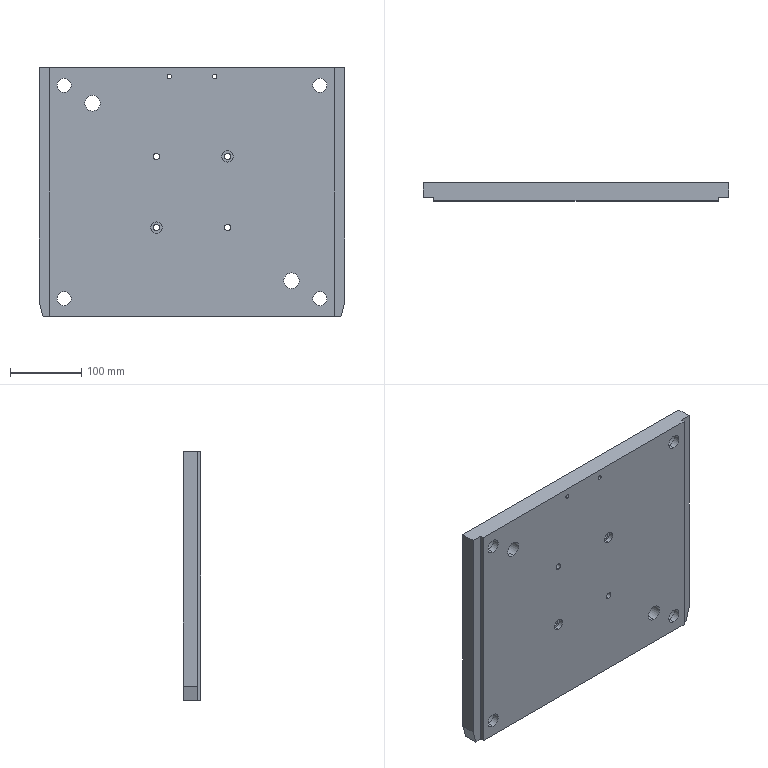Part | STEP file | OP10-104_upper base plate (R) | 1 solid | 66 faces | box 430 x 25 x 350 mm | volume 3618986 mm3 | cylinder 44 | plane 22 | commonest cylinder face diameters 9 x8 15 x8 20 x8 30 x8 6 x4 16 x4